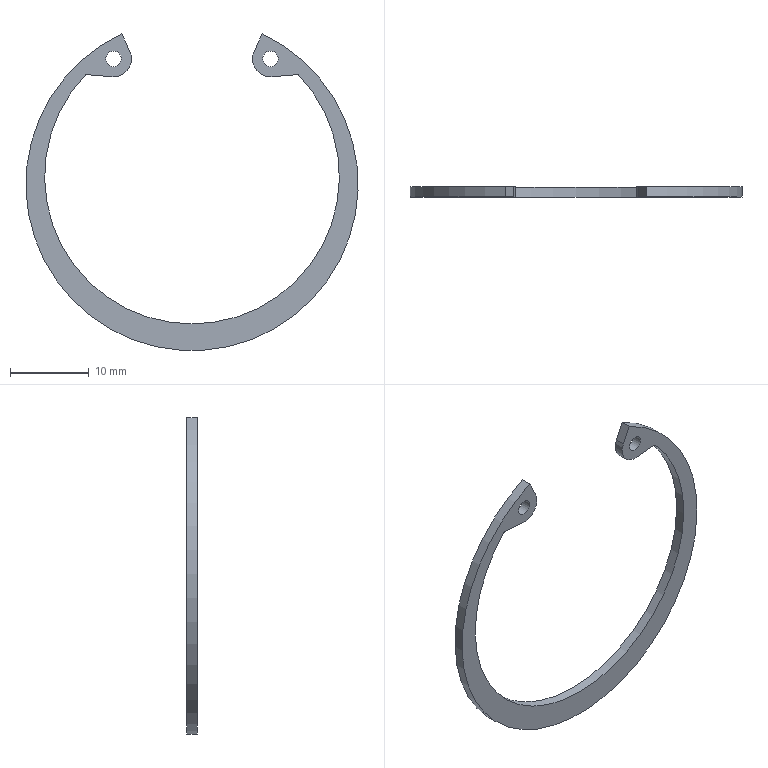Part | NX | features int snap ring 98409A236 2 | 1 solid | 14 faces | box 42.164 x 1.27 x 40.189 mm | volume 371.433 mm3 | cylinder 8 | plane 6 | commonest cylinder face diameters 0.508 x2 1.981 x2 4.572 x2 37.402 x1 42.164 x1
STEP:
#1=CARTESIAN_POINT('',(-8.91,-1.27,19.107));
#2=VERTEX_POINT('',#1);
#3=CARTESIAN_POINT('',(8.91,-1.27,19.107));
#4=VERTEX_POINT('',#3);
#5=CARTESIAN_POINT('',(0.,-1.27,0.));
#6=DIRECTION('',(0.,1.,0.));
#7=DIRECTION('',(0.,0.,1.));
#8=AXIS2_PLACEMENT_3D('',#5,#6,#7);
#9=CIRCLE('',#8,21.082);
#10=EDGE_CURVE('',#2,#4,#9,.F.);
#11=ORIENTED_EDGE('',*,*,#10,.T.);
#12=CARTESIAN_POINT('',(7.885,-1.27,16.909));
#13=VERTEX_POINT('',#12);
#14=CARTESIAN_POINT('',(8.91,-1.27,19.107));
#15=DIRECTION('',(-0.4226,0.,-0.9063));
#16=VECTOR('',#15,1000.);
#17=LINE('',#14,#16);
#18=EDGE_CURVE('',#4,#13,#17,.T.);
#19=ORIENTED_EDGE('',*,*,#18,.T.);
#20=CARTESIAN_POINT('',(10.156,-1.27,13.665));
#21=VERTEX_POINT('',#20);
#22=CARTESIAN_POINT('',(9.956,-1.27,15.942));
#23=DIRECTION('',(0.,1.,0.));
#24=DIRECTION('',(0.,0.,1.));
#25=AXIS2_PLACEMENT_3D('',#22,#23,#24);
#26=CIRCLE('',#25,2.286);
#27=EDGE_CURVE('',#13,#21,#26,.F.);
#28=ORIENTED_EDGE('',*,*,#27,.T.);
#29=CARTESIAN_POINT('',(13.362,-1.27,13.946));
#30=VERTEX_POINT('',#29);
#31=CARTESIAN_POINT('',(10.156,-1.27,13.665));
#32=DIRECTION('',(0.9962,0.,0.08716));
#33=VECTOR('',#32,1000.);
#34=LINE('',#31,#33);
#35=EDGE_CURVE('',#21,#30,#34,.T.);
#36=ORIENTED_EDGE('',*,*,#35,.T.);
#37=CARTESIAN_POINT('',(13.568,-1.27,13.867));
#38=VERTEX_POINT('',#37);
#39=CARTESIAN_POINT('',(13.384,-1.27,13.693));
#40=DIRECTION('',(0.,-1.,0.));
#41=DIRECTION('',(0.,0.,-1.));
#42=AXIS2_PLACEMENT_3D('',#39,#40,#41);
#43=CIRCLE('',#42,0.254);
#44=EDGE_CURVE('',#30,#38,#43,.F.);
#45=ORIENTED_EDGE('',*,*,#44,.T.);
#46=CARTESIAN_POINT('',(-13.568,-1.27,13.867));
#47=VERTEX_POINT('',#46);
#48=CARTESIAN_POINT('',(0.,-1.27,0.9974));
#49=DIRECTION('',(0.,1.,0.));
#50=DIRECTION('',(0.,0.,1.));
#51=AXIS2_PLACEMENT_3D('',#48,#49,#50);
#52=CIRCLE('',#51,18.701);
#53=EDGE_CURVE('',#38,#47,#52,.T.);
#54=ORIENTED_EDGE('',*,*,#53,.T.);
#55=CARTESIAN_POINT('',(-13.362,-1.27,13.946));
#56=VERTEX_POINT('',#55);
#57=CARTESIAN_POINT('',(-13.384,-1.27,13.693));
#58=DIRECTION('',(0.,1.,0.));
#59=DIRECTION('',(0.,0.,1.));
#60=AXIS2_PLACEMENT_3D('',#57,#58,#59);
#61=CIRCLE('',#60,0.254);
#62=EDGE_CURVE('',#47,#56,#61,.T.);
#63=ORIENTED_EDGE('',*,*,#62,.T.);
#64=CARTESIAN_POINT('',(-10.156,-1.27,13.665));
#65=VERTEX_POINT('',#64);
#66=CARTESIAN_POINT('',(-13.362,-1.27,13.946));
#67=DIRECTION('',(0.9962,0.,-0.08716));
#68=VECTOR('',#67,1000.);
#69=LINE('',#66,#68);
#70=EDGE_CURVE('',#56,#65,#69,.T.);
#71=ORIENTED_EDGE('',*,*,#70,.T.);
#72=CARTESIAN_POINT('',(-7.885,-1.27,16.909));
#73=VERTEX_POINT('',#72);
#74=CARTESIAN_POINT('',(-9.956,-1.27,15.942));
#75=DIRECTION('',(0.,1.,0.));
#76=DIRECTION('',(0.,0.,1.));
#77=AXIS2_PLACEMENT_3D('',#74,#75,#76);
#78=CIRCLE('',#77,2.286);
#79=EDGE_CURVE('',#65,#73,#78,.F.);
#80=ORIENTED_EDGE('',*,*,#79,.T.);
#81=CARTESIAN_POINT('',(-7.885,-1.27,16.909));
#82=DIRECTION('',(-0.4226,0.,0.9063));
#83=VECTOR('',#82,1000.);
#84=LINE('',#81,#83);
#85=EDGE_CURVE('',#73,#2,#84,.T.);
#86=ORIENTED_EDGE('',*,*,#85,.T.);
#87=EDGE_LOOP('',(#11,#19,#28,#36,#45,#54,#63,#71,#80,#86));
#88=FACE_BOUND('',#87,.T.);
#89=CARTESIAN_POINT('',(9.956,-1.27,16.933));
#90=VERTEX_POINT('',#89);
#91=CARTESIAN_POINT('',(9.956,-1.27,15.942));
#92=DIRECTION('',(0.,1.,0.));
#93=DIRECTION('',(0.,0.,1.));
#94=AXIS2_PLACEMENT_3D('',#91,#92,#93);
#95=CIRCLE('',#94,0.9906);
#96=EDGE_CURVE('',#90,#90,#95,.T.);
#97=ORIENTED_EDGE('',*,*,#96,.T.);
#98=EDGE_LOOP('',(#97));
#99=FACE_BOUND('',#98,.T.);
#100=CARTESIAN_POINT('',(-9.956,-1.27,16.933));
#101=VERTEX_POINT('',#100);
#102=CARTESIAN_POINT('',(-9.956,-1.27,15.942));
#103=DIRECTION('',(0.,1.,0.));
#104=DIRECTION('',(0.,0.,1.));
#105=AXIS2_PLACEMENT_3D('',#102,#103,#104);
#106=CIRCLE('',#105,0.9906);
#107=EDGE_CURVE('',#101,#101,#106,.T.);
#108=ORIENTED_EDGE('',*,*,#107,.T.);
#109=EDGE_LOOP('',(#108));
#110=FACE_BOUND('',#109,.T.);
#111=CARTESIAN_POINT('',(9.956,-1.27,15.942));
#112=DIRECTION('',(0.,-1.,0.));
#113=DIRECTION('',(0.,0.,-1.));
#114=AXIS2_PLACEMENT_3D('',#111,#112,#113);
#115=PLANE('',#114);
#116=ADVANCED_FACE('',(#88,#99,#110),#115,.T.);
#117=ORIENTED_EDGE('',*,*,#18,.F.);
#118=CARTESIAN_POINT('',(8.91,0.,19.107));
#119=VERTEX_POINT('',#118);
#120=CARTESIAN_POINT('',(8.91,-1.27,19.107));
#121=DIRECTION('',(0.,1.,0.));
#122=VECTOR('',#121,1000.);
#123=LINE('',#120,#122);
#124=EDGE_CURVE('',#4,#119,#123,.T.);
#125=ORIENTED_EDGE('',*,*,#124,.T.);
#126=CARTESIAN_POINT('',(7.885,0.,16.909));
#127=VERTEX_POINT('',#126);
#128=CARTESIAN_POINT('',(8.91,0.,19.107));
#129=DIRECTION('',(0.4226,0.,0.9063));
#130=VECTOR('',#129,1000.);
#131=LINE('',#128,#130);
#132=EDGE_CURVE('',#119,#127,#131,.F.);
#133=ORIENTED_EDGE('',*,*,#132,.T.);
#134=CARTESIAN_POINT('',(7.885,-1.27,16.909));
#135=DIRECTION('',(0.,1.,0.));
#136=VECTOR('',#135,1000.);
#137=LINE('',#134,#136);
#138=EDGE_CURVE('',#127,#13,#137,.F.);
#139=ORIENTED_EDGE('',*,*,#138,.T.);
#140=EDGE_LOOP('',(#117,#125,#133,#139));
#141=FACE_BOUND('',#140,.T.);
#142=CARTESIAN_POINT('',(8.91,-1.27,19.107));
#143=DIRECTION('',(-0.9063,0.,0.4226));
#144=DIRECTION('',(0.4226,0.,0.9063));
#145=AXIS2_PLACEMENT_3D('',#142,#143,#144);
#146=PLANE('',#145);
#147=ADVANCED_FACE('',(#141),#146,.T.);
#148=ORIENTED_EDGE('',*,*,#10,.F.);
#149=CARTESIAN_POINT('',(-8.91,0.,19.107));
#150=VERTEX_POINT('',#149);
#151=CARTESIAN_POINT('',(-8.91,-1.27,19.107));
#152=DIRECTION('',(0.,1.,0.));
#153=VECTOR('',#152,1000.);
#154=LINE('',#151,#153);
#155=EDGE_CURVE('',#2,#150,#154,.T.);
#156=ORIENTED_EDGE('',*,*,#155,.T.);
#157=CARTESIAN_POINT('',(0.,0.,0.));
#158=DIRECTION('',(0.,1.,0.));
#159=DIRECTION('',(0.,0.,1.));
#160=AXIS2_PLACEMENT_3D('',#157,#158,#159);
#161=CIRCLE('',#160,21.082);
#162=EDGE_CURVE('',#150,#119,#161,.F.);
#163=ORIENTED_EDGE('',*,*,#162,.T.);
#164=ORIENTED_EDGE('',*,*,#124,.F.);
#165=EDGE_LOOP('',(#148,#156,#163,#164));
#166=FACE_BOUND('',#165,.T.);
#167=CARTESIAN_POINT('',(0.,-1.27,0.));
#168=DIRECTION('',(0.,1.,0.));
#169=DIRECTION('',(0.,0.,1.));
#170=AXIS2_PLACEMENT_3D('',#167,#168,#169);
#171=CYLINDRICAL_SURFACE('',#170,21.082);
#172=ADVANCED_FACE('',(#166),#171,.T.);
#173=ORIENTED_EDGE('',*,*,#85,.F.);
#174=CARTESIAN_POINT('',(-7.885,0.,16.909));
#175=VERTEX_POINT('',#174);
#176=CARTESIAN_POINT('',(-7.885,-1.27,16.909));
#177=DIRECTION('',(0.,1.,0.));
#178=VECTOR('',#177,1000.);
#179=LINE('',#176,#178);
#180=EDGE_CURVE('',#73,#175,#179,.T.);
#181=ORIENTED_EDGE('',*,*,#180,.T.);
#182=CARTESIAN_POINT('',(-8.91,0.,19.107));
#183=DIRECTION('',(0.4226,0.,-0.9063));
#184=VECTOR('',#183,1000.);
#185=LINE('',#182,#184);
#186=EDGE_CURVE('',#175,#150,#185,.F.);
#187=ORIENTED_EDGE('',*,*,#186,.T.);
#188=ORIENTED_EDGE('',*,*,#155,.F.);
#189=EDGE_LOOP('',(#173,#181,#187,#188));
#190=FACE_BOUND('',#189,.T.);
#191=CARTESIAN_POINT('',(-8.91,-1.27,19.107));
#192=DIRECTION('',(0.9063,0.,0.4226));
#193=DIRECTION('',(0.4226,0.,-0.9063));
#194=AXIS2_PLACEMENT_3D('',#191,#192,#193);
#195=PLANE('',#194);
#196=ADVANCED_FACE('',(#190),#195,.T.);
#197=ORIENTED_EDGE('',*,*,#79,.F.);
#198=CARTESIAN_POINT('',(-10.156,0.,13.665));
#199=VERTEX_POINT('',#198);
#200=CARTESIAN_POINT('',(-10.156,-1.27,13.665));
#201=DIRECTION('',(0.,1.,0.));
#202=VECTOR('',#201,1000.);
#203=LINE('',#200,#202);
#204=EDGE_CURVE('',#65,#199,#203,.T.);
#205=ORIENTED_EDGE('',*,*,#204,.T.);
#206=CARTESIAN_POINT('',(-9.956,0.,15.942));
#207=DIRECTION('',(0.,1.,0.));
#208=DIRECTION('',(0.,0.,1.));
#209=AXIS2_PLACEMENT_3D('',#206,#207,#208);
#210=CIRCLE('',#209,2.286);
#211=EDGE_CURVE('',#199,#175,#210,.F.);
#212=ORIENTED_EDGE('',*,*,#211,.T.);
#213=ORIENTED_EDGE('',*,*,#180,.F.);
#214=EDGE_LOOP('',(#197,#205,#212,#213));
#215=FACE_BOUND('',#214,.T.);
#216=CARTESIAN_POINT('',(-9.956,-1.27,15.942));
#217=DIRECTION('',(0.,1.,0.));
#218=DIRECTION('',(0.,0.,1.));
#219=AXIS2_PLACEMENT_3D('',#216,#217,#218);
#220=CYLINDRICAL_SURFACE('',#219,2.286);
#221=ADVANCED_FACE('',(#215),#220,.T.);
#222=CARTESIAN_POINT('',(-13.362,0.,13.946));
#223=VERTEX_POINT('',#222);
#224=CARTESIAN_POINT('',(-13.483,0.,13.956));
#225=DIRECTION('',(-0.9962,0.,0.08716));
#226=VECTOR('',#225,1000.);
#227=LINE('',#224,#226);
#228=EDGE_CURVE('',#223,#199,#227,.F.);
#229=ORIENTED_EDGE('',*,*,#228,.T.);
#230=ORIENTED_EDGE('',*,*,#204,.F.);
#231=ORIENTED_EDGE('',*,*,#70,.F.);
#232=CARTESIAN_POINT('',(-13.362,-1.27,13.946));
#233=DIRECTION('',(0.,1.,0.));
#234=VECTOR('',#233,1000.);
#235=LINE('',#232,#234);
#236=EDGE_CURVE('',#56,#223,#235,.T.);
#237=ORIENTED_EDGE('',*,*,#236,.T.);
#238=EDGE_LOOP('',(#229,#230,#231,#237));
#239=FACE_BOUND('',#238,.T.);
#240=CARTESIAN_POINT('',(-13.483,-1.27,13.956));
#241=DIRECTION('',(-0.08716,0.,-0.9962));
#242=DIRECTION('',(-0.9962,0.,0.08716));
#243=AXIS2_PLACEMENT_3D('',#240,#241,#242);
#244=PLANE('',#243);
#245=ADVANCED_FACE('',(#239),#244,.T.);
#246=ORIENTED_EDGE('',*,*,#236,.F.);
#247=ORIENTED_EDGE('',*,*,#62,.F.);
#248=CARTESIAN_POINT('',(-13.568,0.,13.867));
#249=VERTEX_POINT('',#248);
#250=CARTESIAN_POINT('',(-13.568,-1.27,13.867));
#251=DIRECTION('',(0.,1.,0.));
#252=VECTOR('',#251,1000.);
#253=LINE('',#250,#252);
#254=EDGE_CURVE('',#249,#47,#253,.F.);
#255=ORIENTED_EDGE('',*,*,#254,.F.);
#256=CARTESIAN_POINT('',(-13.384,0.,13.693));
#257=DIRECTION('',(0.,-1.,0.));
#258=DIRECTION('',(0.,0.,-1.));
#259=AXIS2_PLACEMENT_3D('',#256,#257,#258);
#260=CIRCLE('',#259,0.254);
#261=EDGE_CURVE('',#223,#249,#260,.T.);
#262=ORIENTED_EDGE('',*,*,#261,.F.);
#263=EDGE_LOOP('',(#246,#247,#255,#262));
#264=FACE_BOUND('',#263,.T.);
#265=CARTESIAN_POINT('',(-13.384,-1.27,13.693));
#266=DIRECTION('',(0.,1.,0.));
#267=DIRECTION('',(0.,0.,1.));
#268=AXIS2_PLACEMENT_3D('',#265,#266,#267);
#269=CYLINDRICAL_SURFACE('',#268,0.254);
#270=ADVANCED_FACE('',(#264),#269,.F.);
#271=ORIENTED_EDGE('',*,*,#254,.T.);
#272=ORIENTED_EDGE('',*,*,#53,.F.);
#273=CARTESIAN_POINT('',(13.568,0.,13.867));
#274=VERTEX_POINT('',#273);
#275=CARTESIAN_POINT('',(13.568,-1.27,13.867));
#276=DIRECTION('',(0.,1.,0.));
#277=VECTOR('',#276,1000.);
#278=LINE('',#275,#277);
#279=EDGE_CURVE('',#274,#38,#278,.F.);
#280=ORIENTED_EDGE('',*,*,#279,.F.);
#281=CARTESIAN_POINT('',(0.,0.,0.9974));
#282=DIRECTION('',(0.,1.,0.));
#283=DIRECTION('',(0.,0.,1.));
#284=AXIS2_PLACEMENT_3D('',#281,#282,#283);
#285=CIRCLE('',#284,18.701);
#286=EDGE_CURVE('',#249,#274,#285,.F.);
#287=ORIENTED_EDGE('',*,*,#286,.F.);
#288=EDGE_LOOP('',(#271,#272,#280,#287));
#289=FACE_BOUND('',#288,.T.);
#290=CARTESIAN_POINT('',(0.,-1.27,0.9974));
#291=DIRECTION('',(0.,1.,0.));
#292=DIRECTION('',(0.,0.,1.));
#293=AXIS2_PLACEMENT_3D('',#290,#291,#292);
#294=CYLINDRICAL_SURFACE('',#293,18.701);
#295=ADVANCED_FACE('',(#289),#294,.F.);
#296=ORIENTED_EDGE('',*,*,#279,.T.);
#297=ORIENTED_EDGE('',*,*,#44,.F.);
#298=CARTESIAN_POINT('',(13.362,0.,13.946));
#299=VERTEX_POINT('',#298);
#300=CARTESIAN_POINT('',(13.362,-1.27,13.946));
#301=DIRECTION('',(0.,1.,0.));
#302=VECTOR('',#301,1000.);
#303=LINE('',#300,#302);
#304=EDGE_CURVE('',#299,#30,#303,.F.);
#305=ORIENTED_EDGE('',*,*,#304,.F.);
#306=CARTESIAN_POINT('',(13.384,0.,13.693));
#307=DIRECTION('',(0.,1.,0.));
#308=DIRECTION('',(0.,0.,1.));
#309=AXIS2_PLACEMENT_3D('',#306,#307,#308);
#310=CIRCLE('',#309,0.254);
#311=EDGE_CURVE('',#274,#299,#310,.F.);
#312=ORIENTED_EDGE('',*,*,#311,.F.);
#313=EDGE_LOOP('',(#296,#297,#305,#312));
#314=FACE_BOUND('',#313,.T.);
#315=CARTESIAN_POINT('',(13.384,-1.27,13.693));
#316=DIRECTION('',(0.,1.,0.));
#317=DIRECTION('',(0.,0.,1.));
#318=AXIS2_PLACEMENT_3D('',#315,#316,#317);
#319=CYLINDRICAL_SURFACE('',#318,0.254);
#320=ADVANCED_FACE('',(#314),#319,.F.);
#321=ORIENTED_EDGE('',*,*,#35,.F.);
#322=CARTESIAN_POINT('',(10.156,0.,13.665));
#323=VERTEX_POINT('',#322);
#324=CARTESIAN_POINT('',(10.156,-1.27,13.665));
#325=DIRECTION('',(0.,1.,0.));
#326=VECTOR('',#325,1000.);
#327=LINE('',#324,#326);
#328=EDGE_CURVE('',#21,#323,#327,.T.);
#329=ORIENTED_EDGE('',*,*,#328,.T.);
#330=CARTESIAN_POINT('',(13.483,0.,13.956));
#331=DIRECTION('',(-0.9962,0.,-0.08716));
#332=VECTOR('',#331,1000.);
#333=LINE('',#330,#332);
#334=EDGE_CURVE('',#323,#299,#333,.F.);
#335=ORIENTED_EDGE('',*,*,#334,.T.);
#336=ORIENTED_EDGE('',*,*,#304,.T.);
#337=EDGE_LOOP('',(#321,#329,#335,#336));
#338=FACE_BOUND('',#337,.T.);
#339=CARTESIAN_POINT('',(13.483,-1.27,13.956));
#340=DIRECTION('',(0.08716,0.,-0.9962));
#341=DIRECTION('',(-0.9962,0.,-0.08716));
#342=AXIS2_PLACEMENT_3D('',#339,#340,#341);
#343=PLANE('',#342);
#344=ADVANCED_FACE('',(#338),#343,.T.);
#345=ORIENTED_EDGE('',*,*,#27,.F.);
#346=ORIENTED_EDGE('',*,*,#138,.F.);
#347=CARTESIAN_POINT('',(9.956,0.,15.942));
#348=DIRECTION('',(0.,1.,0.));
#349=DIRECTION('',(0.,0.,1.));
#350=AXIS2_PLACEMENT_3D('',#347,#348,#349);
#351=CIRCLE('',#350,2.286);
#352=EDGE_CURVE('',#127,#323,#351,.F.);
#353=ORIENTED_EDGE('',*,*,#352,.T.);
#354=ORIENTED_EDGE('',*,*,#328,.F.);
#355=EDGE_LOOP('',(#345,#346,#353,#354));
#356=FACE_BOUND('',#355,.T.);
#357=CARTESIAN_POINT('',(9.956,-1.27,15.942));
#358=DIRECTION('',(0.,1.,0.));
#359=DIRECTION('',(0.,0.,1.));
#360=AXIS2_PLACEMENT_3D('',#357,#358,#359);
#361=CYLINDRICAL_SURFACE('',#360,2.286);
#362=ADVANCED_FACE('',(#356),#361,.T.);
#363=CARTESIAN_POINT('',(9.956,0.,16.933));
#364=VERTEX_POINT('',#363);
#365=CARTESIAN_POINT('',(9.956,0.,15.942));
#366=DIRECTION('',(0.,1.,0.));
#367=DIRECTION('',(0.,0.,1.));
#368=AXIS2_PLACEMENT_3D('',#365,#366,#367);
#369=CIRCLE('',#368,0.9906);
#370=EDGE_CURVE('',#364,#364,#369,.F.);
#371=ORIENTED_EDGE('',*,*,#370,.F.);
#372=EDGE_LOOP('',(#371));
#373=FACE_BOUND('',#372,.T.);
#374=ORIENTED_EDGE('',*,*,#96,.F.);
#375=EDGE_LOOP('',(#374));
#376=FACE_BOUND('',#375,.T.);
#377=CARTESIAN_POINT('',(9.956,-1.27,15.942));
#378=DIRECTION('',(0.,1.,0.));
#379=DIRECTION('',(0.,0.,1.));
#380=AXIS2_PLACEMENT_3D('',#377,#378,#379);
#381=CYLINDRICAL_SURFACE('',#380,0.9906);
#382=ADVANCED_FACE('',(#373,#376),#381,.F.);
#383=CARTESIAN_POINT('',(-9.956,0.,16.933));
#384=VERTEX_POINT('',#383);
#385=CARTESIAN_POINT('',(-9.956,0.,15.942));
#386=DIRECTION('',(0.,1.,0.));
#387=DIRECTION('',(0.,0.,1.));
#388=AXIS2_PLACEMENT_3D('',#385,#386,#387);
#389=CIRCLE('',#388,0.9906);
#390=EDGE_CURVE('',#384,#384,#389,.F.);
#391=ORIENTED_EDGE('',*,*,#390,.F.);
#392=EDGE_LOOP('',(#391));
#393=FACE_BOUND('',#392,.T.);
#394=ORIENTED_EDGE('',*,*,#107,.F.);
#395=EDGE_LOOP('',(#394));
#396=FACE_BOUND('',#395,.T.);
#397=CARTESIAN_POINT('',(-9.956,-1.27,15.942));
#398=DIRECTION('',(0.,1.,0.));
#399=DIRECTION('',(0.,0.,1.));
#400=AXIS2_PLACEMENT_3D('',#397,#398,#399);
#401=CYLINDRICAL_SURFACE('',#400,0.9906);
#402=ADVANCED_FACE('',(#393,#396),#401,.F.);
#403=ORIENTED_EDGE('',*,*,#132,.F.);
#404=ORIENTED_EDGE('',*,*,#162,.F.);
#405=ORIENTED_EDGE('',*,*,#186,.F.);
#406=ORIENTED_EDGE('',*,*,#211,.F.);
#407=ORIENTED_EDGE('',*,*,#228,.F.);
#408=ORIENTED_EDGE('',*,*,#261,.T.);
#409=ORIENTED_EDGE('',*,*,#286,.T.);
#410=ORIENTED_EDGE('',*,*,#311,.T.);
#411=ORIENTED_EDGE('',*,*,#334,.F.);
#412=ORIENTED_EDGE('',*,*,#352,.F.);
#413=EDGE_LOOP('',(#403,#404,#405,#406,#407,#408,#409,#410,#411,#412));
#414=FACE_BOUND('',#413,.T.);
#415=ORIENTED_EDGE('',*,*,#370,.T.);
#416=EDGE_LOOP('',(#415));
#417=FACE_BOUND('',#416,.T.);
#418=ORIENTED_EDGE('',*,*,#390,.T.);
#419=EDGE_LOOP('',(#418));
#420=FACE_BOUND('',#419,.T.);
#421=CARTESIAN_POINT('',(9.956,0.,15.942));
#422=DIRECTION('',(0.,-1.,0.));
#423=DIRECTION('',(0.,0.,-1.));
#424=AXIS2_PLACEMENT_3D('',#421,#422,#423);
#425=PLANE('',#424);
#426=ADVANCED_FACE('',(#414,#417,#420),#425,.F.);
#427=CLOSED_SHELL('',(#116,#147,#172,#196,#221,#245,#270,#295,#320,#344,#362,#382,#402,#426));
#428=MANIFOLD_SOLID_BREP('',#427);
#429=(LENGTH_UNIT()NAMED_UNIT(*)SI_UNIT(.MILLI.,.METRE.));
#430=UNCERTAINTY_MEASURE_WITH_UNIT(LENGTH_MEASURE(0.00001),#429,'','');
#431=(NAMED_UNIT(*)PLANE_ANGLE_UNIT()SI_UNIT($,.RADIAN.));
#432=(NAMED_UNIT(*)SI_UNIT($,.STERADIAN.)SOLID_ANGLE_UNIT());
#433=(GEOMETRIC_REPRESENTATION_CONTEXT(3)GLOBAL_UNCERTAINTY_ASSIGNED_CONTEXT((#430))GLOBAL_UNIT_ASSIGNED_CONTEXT((#429,#431,#432))REPRESENTATION_CONTEXT('',''));
#434=ADVANCED_BREP_SHAPE_REPRESENTATION('',(#428),#433);